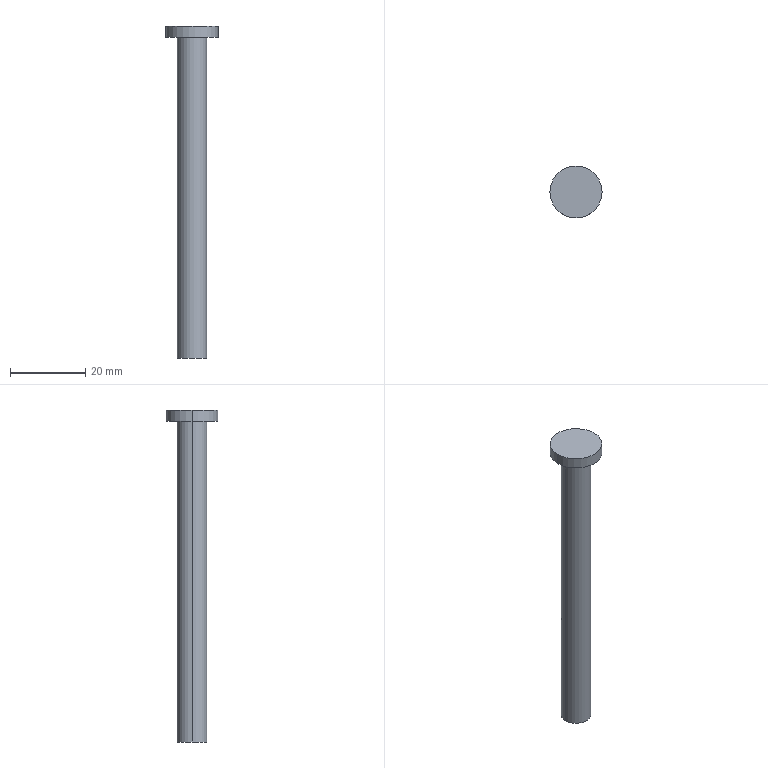Part | SolidWorks | features Extrusion 1, ICE 1 | 1 solid | 7 faces | box 13.8 x 13.8 x 88 mm | volume 4510 mm3 | cylinder 4 | plane 3 | commonest cylinder face diameters 7.8 x2 13.8 x2
STEP:
#1=CARTESIAN_POINT('',(6.287,-35.,35.));
#2=VERTEX_POINT('',#1);
#3=CARTESIAN_POINT('',(-7.513,-35.,35.));
#4=VERTEX_POINT('',#3);
#5=CARTESIAN_POINT('',(-0.6135,-35.,35.));
#6=DIRECTION('',(0.,0.,1.));
#7=DIRECTION('',(-1.,0.,0.));
#8=AXIS2_PLACEMENT_3D('',#5,#6,#7);
#9=CIRCLE('',#8,6.9);
#10=EDGE_CURVE('',#2,#4,#9,.T.);
#11=ORIENTED_EDGE('',*,*,#10,.T.);
#12=CARTESIAN_POINT('',(-7.513,-35.,38.));
#13=VERTEX_POINT('',#12);
#14=CARTESIAN_POINT('',(-7.513,-35.,15.484));
#15=DIRECTION('',(0.,0.,1.));
#16=VECTOR('',#15,1000.);
#17=LINE('',#14,#16);
#18=EDGE_CURVE('',#4,#13,#17,.T.);
#19=ORIENTED_EDGE('',*,*,#18,.T.);
#20=CARTESIAN_POINT('',(6.287,-35.,38.));
#21=VERTEX_POINT('',#20);
#22=CARTESIAN_POINT('',(-0.6135,-35.,38.));
#23=DIRECTION('',(0.,0.,1.));
#24=DIRECTION('',(1.,0.,0.));
#25=AXIS2_PLACEMENT_3D('',#22,#23,#24);
#26=CIRCLE('',#25,6.9);
#27=EDGE_CURVE('',#21,#13,#26,.T.);
#28=ORIENTED_EDGE('',*,*,#27,.F.);
#29=CARTESIAN_POINT('',(6.287,-35.,15.484));
#30=DIRECTION('',(0.,0.,1.));
#31=VECTOR('',#30,1000.);
#32=LINE('',#29,#31);
#33=EDGE_CURVE('',#2,#21,#32,.T.);
#34=ORIENTED_EDGE('',*,*,#33,.F.);
#35=EDGE_LOOP('',(#11,#19,#28,#34));
#36=FACE_OUTER_BOUND('',#35,.T.);
#37=CARTESIAN_POINT('',(-0.6135,-35.,15.484));
#38=DIRECTION('',(0.,0.,1.));
#39=DIRECTION('',(1.,0.,0.));
#40=AXIS2_PLACEMENT_3D('',#37,#38,#39);
#41=CYLINDRICAL_SURFACE('',#40,6.9);
#42=ADVANCED_FACE('',(#36),#41,.T.);
#43=CARTESIAN_POINT('',(-4.513,-35.,35.));
#44=VERTEX_POINT('',#43);
#45=CARTESIAN_POINT('',(3.287,-35.,35.));
#46=VERTEX_POINT('',#45);
#47=CARTESIAN_POINT('',(-0.6135,-35.,35.));
#48=DIRECTION('',(0.,0.,-1.));
#49=DIRECTION('',(-1.,0.,0.));
#50=AXIS2_PLACEMENT_3D('',#47,#48,#49);
#51=CIRCLE('',#50,3.9);
#52=EDGE_CURVE('',#44,#46,#51,.T.);
#53=ORIENTED_EDGE('',*,*,#52,.T.);
#54=CARTESIAN_POINT('',(3.287,-35.,-50.));
#55=VERTEX_POINT('',#54);
#56=CARTESIAN_POINT('',(3.287,-35.,38.));
#57=DIRECTION('',(0.,0.,-1.));
#58=VECTOR('',#57,1000.);
#59=LINE('',#56,#58);
#60=EDGE_CURVE('',#46,#55,#59,.T.);
#61=ORIENTED_EDGE('',*,*,#60,.T.);
#62=CARTESIAN_POINT('',(-4.513,-35.,-50.));
#63=VERTEX_POINT('',#62);
#64=CARTESIAN_POINT('',(-0.6135,-35.,-50.));
#65=DIRECTION('',(0.,0.,1.));
#66=DIRECTION('',(1.,0.,0.));
#67=AXIS2_PLACEMENT_3D('',#64,#65,#66);
#68=CIRCLE('',#67,3.9);
#69=EDGE_CURVE('',#55,#63,#68,.T.);
#70=ORIENTED_EDGE('',*,*,#69,.T.);
#71=CARTESIAN_POINT('',(-4.513,-35.,38.));
#72=DIRECTION('',(0.,0.,-1.));
#73=VECTOR('',#72,1000.);
#74=LINE('',#71,#73);
#75=EDGE_CURVE('',#44,#63,#74,.T.);
#76=ORIENTED_EDGE('',*,*,#75,.F.);
#77=EDGE_LOOP('',(#53,#61,#70,#76));
#78=FACE_OUTER_BOUND('',#77,.T.);
#79=CARTESIAN_POINT('',(-0.6135,-35.,38.));
#80=DIRECTION('',(0.,0.,-1.));
#81=DIRECTION('',(-1.,0.,0.));
#82=AXIS2_PLACEMENT_3D('',#79,#80,#81);
#83=CYLINDRICAL_SURFACE('',#82,3.9);
#84=ADVANCED_FACE('',(#78),#83,.T.);
#85=ORIENTED_EDGE('',*,*,#60,.F.);
#86=CARTESIAN_POINT('',(-0.6135,-35.,35.));
#87=DIRECTION('',(0.,0.,-1.));
#88=DIRECTION('',(-1.,0.,0.));
#89=AXIS2_PLACEMENT_3D('',#86,#87,#88);
#90=CIRCLE('',#89,3.9);
#91=EDGE_CURVE('',#46,#44,#90,.T.);
#92=ORIENTED_EDGE('',*,*,#91,.T.);
#93=ORIENTED_EDGE('',*,*,#75,.T.);
#94=CARTESIAN_POINT('',(-0.6135,-35.,-50.));
#95=DIRECTION('',(0.,0.,1.));
#96=DIRECTION('',(1.,0.,0.));
#97=AXIS2_PLACEMENT_3D('',#94,#95,#96);
#98=CIRCLE('',#97,3.9);
#99=EDGE_CURVE('',#63,#55,#98,.T.);
#100=ORIENTED_EDGE('',*,*,#99,.T.);
#101=EDGE_LOOP('',(#85,#92,#93,#100));
#102=FACE_OUTER_BOUND('',#101,.T.);
#103=CARTESIAN_POINT('',(-0.6135,-35.,38.));
#104=DIRECTION('',(0.,0.,-1.));
#105=DIRECTION('',(-1.,0.,0.));
#106=AXIS2_PLACEMENT_3D('',#103,#104,#105);
#107=CYLINDRICAL_SURFACE('',#106,3.9);
#108=ADVANCED_FACE('',(#102),#107,.T.);
#109=ORIENTED_EDGE('',*,*,#99,.F.);
#110=ORIENTED_EDGE('',*,*,#69,.F.);
#111=EDGE_LOOP('',(#109,#110));
#112=FACE_OUTER_BOUND('',#111,.T.);
#113=CARTESIAN_POINT('',(-0.6135,-35.,-50.));
#114=DIRECTION('',(0.,0.,1.));
#115=DIRECTION('',(1.,0.,0.));
#116=AXIS2_PLACEMENT_3D('',#113,#114,#115);
#117=PLANE('',#116);
#118=ADVANCED_FACE('',(#112),#117,.F.);
#119=ORIENTED_EDGE('',*,*,#52,.F.);
#120=ORIENTED_EDGE('',*,*,#91,.F.);
#121=EDGE_LOOP('',(#119,#120));
#122=FACE_BOUND('',#121,.T.);
#123=ORIENTED_EDGE('',*,*,#10,.F.);
#124=CARTESIAN_POINT('',(-0.6135,-35.,35.));
#125=DIRECTION('',(0.,0.,1.));
#126=DIRECTION('',(-1.,0.,0.));
#127=AXIS2_PLACEMENT_3D('',#124,#125,#126);
#128=CIRCLE('',#127,6.9);
#129=EDGE_CURVE('',#4,#2,#128,.T.);
#130=ORIENTED_EDGE('',*,*,#129,.F.);
#131=EDGE_LOOP('',(#123,#130));
#132=FACE_OUTER_BOUND('',#131,.T.);
#133=CARTESIAN_POINT('',(34.387,-70.,35.));
#134=DIRECTION('',(0.,0.,-1.));
#135=DIRECTION('',(0.,1.,0.));
#136=AXIS2_PLACEMENT_3D('',#133,#134,#135);
#137=PLANE('',#136);
#138=ADVANCED_FACE('',(#122,#132),#137,.T.);
#139=ORIENTED_EDGE('',*,*,#18,.F.);
#140=ORIENTED_EDGE('',*,*,#129,.T.);
#141=ORIENTED_EDGE('',*,*,#33,.T.);
#142=CARTESIAN_POINT('',(-0.6135,-35.,38.));
#143=DIRECTION('',(0.,0.,1.));
#144=DIRECTION('',(1.,0.,0.));
#145=AXIS2_PLACEMENT_3D('',#142,#143,#144);
#146=CIRCLE('',#145,6.9);
#147=EDGE_CURVE('',#13,#21,#146,.T.);
#148=ORIENTED_EDGE('',*,*,#147,.F.);
#149=EDGE_LOOP('',(#139,#140,#141,#148));
#150=FACE_OUTER_BOUND('',#149,.T.);
#151=CARTESIAN_POINT('',(-0.6135,-35.,15.484));
#152=DIRECTION('',(0.,0.,1.));
#153=DIRECTION('',(1.,0.,0.));
#154=AXIS2_PLACEMENT_3D('',#151,#152,#153);
#155=CYLINDRICAL_SURFACE('',#154,6.9);
#156=ADVANCED_FACE('',(#150),#155,.T.);
#157=ORIENTED_EDGE('',*,*,#27,.T.);
#158=ORIENTED_EDGE('',*,*,#147,.T.);
#159=EDGE_LOOP('',(#157,#158));
#160=FACE_OUTER_BOUND('',#159,.T.);
#161=CARTESIAN_POINT('',(-0.6135,-35.,38.));
#162=DIRECTION('',(0.,0.,1.));
#163=DIRECTION('',(1.,0.,0.));
#164=AXIS2_PLACEMENT_3D('',#161,#162,#163);
#165=PLANE('',#164);
#166=ADVANCED_FACE('',(#160),#165,.T.);
#167=CLOSED_SHELL('',(#42,#84,#108,#118,#138,#156,#166));
#168=MANIFOLD_SOLID_BREP('',#167);
#169=CARTESIAN_POINT('',(0.,0.,0.));
#170=DIRECTION('',(0.,0.,1.));
#171=DIRECTION('',(1.,0.,0.));
#172=AXIS2_PLACEMENT_3D('',#169,#170,#171);
#173=(LENGTH_UNIT()NAMED_UNIT(*)SI_UNIT(.MILLI.,.METRE.));
#174=UNCERTAINTY_MEASURE_WITH_UNIT(LENGTH_MEASURE(0.00001),#173,'','');
#175=(NAMED_UNIT(*)PLANE_ANGLE_UNIT()SI_UNIT($,.RADIAN.));
#176=(NAMED_UNIT(*)SI_UNIT($,.STERADIAN.)SOLID_ANGLE_UNIT());
#177=(GEOMETRIC_REPRESENTATION_CONTEXT(3)GLOBAL_UNCERTAINTY_ASSIGNED_CONTEXT((#174))GLOBAL_UNIT_ASSIGNED_CONTEXT((#173,#175,#176))REPRESENTATION_CONTEXT('',''));
#178=ADVANCED_BREP_SHAPE_REPRESENTATION('',(#168,#172),#177);